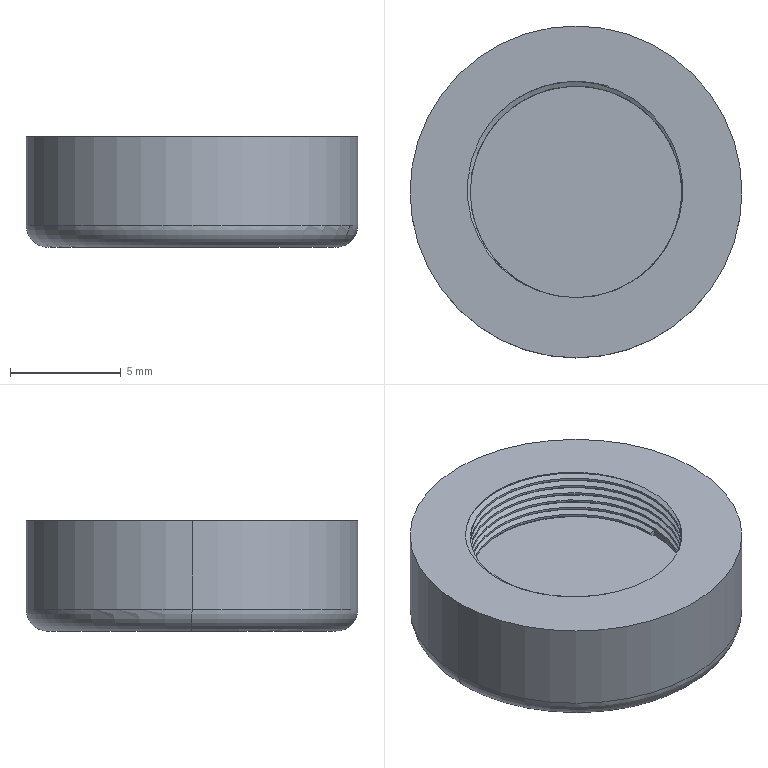Part | SolidWorks | features ICE 2, Extrusion 1, Fillet 1, SweepThread 1 | 1 solid | 73 faces | box 15 x 15 x 5 mm | volume 677.673 mm3 | plane 33 | spline 23 | cylinder 15 | torus 2 | commonest cylinder face diameters 10 x13 15 x2